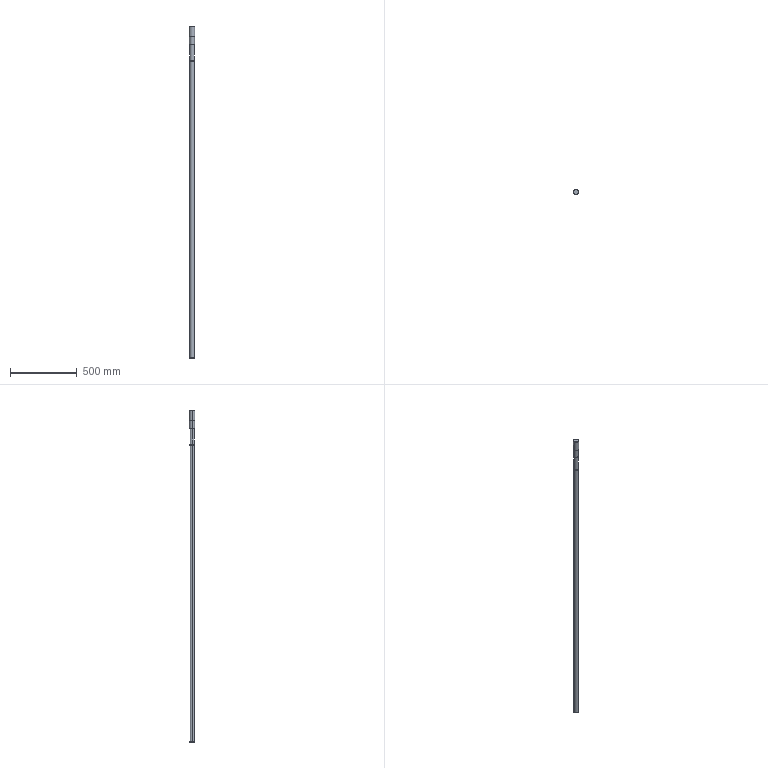Part | SolidWorks | features Chamfer 6, ICE 6, Extrusion 1, MoveFace 1 | 2 solids | 41 faces | box 40 x 40 x 2490 mm | volume 2423592 mm3 | cone 16 | cylinder 15 | plane 10 | commonest cylinder face diameters 16 x4 35 x4 12 x3 38 x2 40 x2
STEP:
#1=CARTESIAN_POINT('',(-7.5,0.,946.05));
#2=VERTEX_POINT('',#1);
#3=CARTESIAN_POINT('',(7.5,0.,946.05));
#4=VERTEX_POINT('',#3);
#5=CARTESIAN_POINT('',(0.,0.,946.05));
#6=DIRECTION('',(0.,0.,-1.));
#7=DIRECTION('',(-1.,0.,0.));
#8=AXIS2_PLACEMENT_3D('',#5,#6,#7);
#9=CIRCLE('',#8,7.5);
#10=EDGE_CURVE('',#2,#4,#9,.T.);
#11=ORIENTED_EDGE('',*,*,#10,.F.);
#12=CARTESIAN_POINT('',(-8.,0.,946.55));
#13=VERTEX_POINT('',#12);
#14=CARTESIAN_POINT('',(-7.5,0.,946.05));
#15=DIRECTION('',(-0.7071,0.,0.7071));
#16=VECTOR('',#15,1000.);
#17=LINE('',#14,#16);
#18=EDGE_CURVE('',#2,#13,#17,.T.);
#19=ORIENTED_EDGE('',*,*,#18,.T.);
#20=CARTESIAN_POINT('',(8.,0.,946.55));
#21=VERTEX_POINT('',#20);
#22=CARTESIAN_POINT('',(0.,0.,946.55));
#23=DIRECTION('',(0.,0.,1.));
#24=DIRECTION('',(-1.,0.,0.));
#25=AXIS2_PLACEMENT_3D('',#22,#23,#24);
#26=CIRCLE('',#25,8.);
#27=EDGE_CURVE('',#21,#13,#26,.T.);
#28=ORIENTED_EDGE('',*,*,#27,.F.);
#29=CARTESIAN_POINT('',(7.5,0.,946.05));
#30=DIRECTION('',(0.7071,0.,0.7071));
#31=VECTOR('',#30,1000.);
#32=LINE('',#29,#31);
#33=EDGE_CURVE('',#4,#21,#32,.T.);
#34=ORIENTED_EDGE('',*,*,#33,.F.);
#35=EDGE_LOOP('',(#11,#19,#28,#34));
#36=FACE_OUTER_BOUND('',#35,.T.);
#37=CARTESIAN_POINT('',(0.,0.,946.05));
#38=DIRECTION('',(0.,0.,1.));
#39=DIRECTION('',(1.,0.,0.));
#40=AXIS2_PLACEMENT_3D('',#37,#38,#39);
#41=CONICAL_SURFACE('',#40,7.5,0.7854);
#42=ADVANCED_FACE('',(#36),#41,.T.);
#43=CARTESIAN_POINT('',(-8.,0.,984.55));
#44=VERTEX_POINT('',#43);
#45=CARTESIAN_POINT('',(8.,0.,984.55));
#46=VERTEX_POINT('',#45);
#47=CARTESIAN_POINT('',(0.,0.,984.55));
#48=DIRECTION('',(0.,0.,-1.));
#49=DIRECTION('',(1.,0.,0.));
#50=AXIS2_PLACEMENT_3D('',#47,#48,#49);
#51=CIRCLE('',#50,8.);
#52=EDGE_CURVE('',#44,#46,#51,.T.);
#53=ORIENTED_EDGE('',*,*,#52,.F.);
#54=CARTESIAN_POINT('',(-8.5,0.,985.05));
#55=VERTEX_POINT('',#54);
#56=CARTESIAN_POINT('',(-8.,0.,984.55));
#57=DIRECTION('',(-0.7071,0.,0.7071));
#58=VECTOR('',#57,1000.);
#59=LINE('',#56,#58);
#60=EDGE_CURVE('',#44,#55,#59,.T.);
#61=ORIENTED_EDGE('',*,*,#60,.T.);
#62=CARTESIAN_POINT('',(8.5,0.,985.05));
#63=VERTEX_POINT('',#62);
#64=CARTESIAN_POINT('',(0.,0.,985.05));
#65=DIRECTION('',(0.,0.,1.));
#66=DIRECTION('',(1.,0.,0.));
#67=AXIS2_PLACEMENT_3D('',#64,#65,#66);
#68=CIRCLE('',#67,8.5);
#69=EDGE_CURVE('',#63,#55,#68,.T.);
#70=ORIENTED_EDGE('',*,*,#69,.F.);
#71=CARTESIAN_POINT('',(8.,0.,984.55));
#72=DIRECTION('',(0.7071,0.,0.7071));
#73=VECTOR('',#72,1000.);
#74=LINE('',#71,#73);
#75=EDGE_CURVE('',#46,#63,#74,.T.);
#76=ORIENTED_EDGE('',*,*,#75,.F.);
#77=EDGE_LOOP('',(#53,#61,#70,#76));
#78=FACE_OUTER_BOUND('',#77,.T.);
#79=CARTESIAN_POINT('',(0.,0.,984.55));
#80=DIRECTION('',(0.,0.,1.));
#81=DIRECTION('',(1.,0.,0.));
#82=AXIS2_PLACEMENT_3D('',#79,#80,#81);
#83=CONICAL_SURFACE('',#82,8.,0.7854);
#84=ADVANCED_FACE('',(#78),#83,.T.);
#85=ORIENTED_EDGE('',*,*,#27,.T.);
#86=CARTESIAN_POINT('',(-8.,0.,946.05));
#87=DIRECTION('',(0.,0.,1.));
#88=VECTOR('',#87,1000.);
#89=LINE('',#86,#88);
#90=EDGE_CURVE('',#13,#44,#89,.T.);
#91=ORIENTED_EDGE('',*,*,#90,.T.);
#92=ORIENTED_EDGE('',*,*,#52,.T.);
#93=CARTESIAN_POINT('',(8.,0.,946.05));
#94=DIRECTION('',(0.,0.,1.));
#95=VECTOR('',#94,1000.);
#96=LINE('',#93,#95);
#97=EDGE_CURVE('',#21,#46,#96,.T.);
#98=ORIENTED_EDGE('',*,*,#97,.F.);
#99=EDGE_LOOP('',(#85,#91,#92,#98));
#100=FACE_OUTER_BOUND('',#99,.T.);
#101=CARTESIAN_POINT('',(0.,0.,946.05));
#102=DIRECTION('',(0.,0.,1.));
#103=DIRECTION('',(1.,0.,0.));
#104=AXIS2_PLACEMENT_3D('',#101,#102,#103);
#105=CYLINDRICAL_SURFACE('',#104,8.);
#106=ADVANCED_FACE('',(#100),#105,.T.);
#107=CARTESIAN_POINT('',(-13.5,0.,985.05));
#108=VERTEX_POINT('',#107);
#109=CARTESIAN_POINT('',(13.5,0.,985.05));
#110=VERTEX_POINT('',#109);
#111=CARTESIAN_POINT('',(0.,0.,985.05));
#112=DIRECTION('',(0.,0.,-1.));
#113=DIRECTION('',(1.,0.,0.));
#114=AXIS2_PLACEMENT_3D('',#111,#112,#113);
#115=CIRCLE('',#114,13.5);
#116=EDGE_CURVE('',#108,#110,#115,.T.);
#117=ORIENTED_EDGE('',*,*,#116,.F.);
#118=CARTESIAN_POINT('',(-17.5,0.,989.05));
#119=VERTEX_POINT('',#118);
#120=CARTESIAN_POINT('',(-17.5,0.,989.05));
#121=DIRECTION('',(-0.7071,0.,0.7071));
#122=VECTOR('',#121,1000.);
#123=LINE('',#120,#122);
#124=EDGE_CURVE('',#108,#119,#123,.T.);
#125=ORIENTED_EDGE('',*,*,#124,.T.);
#126=CARTESIAN_POINT('',(17.5,0.,989.05));
#127=VERTEX_POINT('',#126);
#128=CARTESIAN_POINT('',(0.,0.,989.05));
#129=DIRECTION('',(0.,0.,1.));
#130=DIRECTION('',(1.,0.,0.));
#131=AXIS2_PLACEMENT_3D('',#128,#129,#130);
#132=CIRCLE('',#131,17.5);
#133=EDGE_CURVE('',#127,#119,#132,.T.);
#134=ORIENTED_EDGE('',*,*,#133,.F.);
#135=CARTESIAN_POINT('',(17.5,0.,989.05));
#136=DIRECTION('',(0.7071,0.,0.7071));
#137=VECTOR('',#136,1000.);
#138=LINE('',#135,#137);
#139=EDGE_CURVE('',#110,#127,#138,.T.);
#140=ORIENTED_EDGE('',*,*,#139,.F.);
#141=EDGE_LOOP('',(#117,#125,#134,#140));
#142=FACE_OUTER_BOUND('',#141,.T.);
#143=CARTESIAN_POINT('',(0.,0.,989.05));
#144=DIRECTION('',(0.,0.,1.));
#145=DIRECTION('',(1.,0.,0.));
#146=AXIS2_PLACEMENT_3D('',#143,#144,#145);
#147=CONICAL_SURFACE('',#146,17.5,0.7854);
#148=ADVANCED_FACE('',(#142),#147,.T.);
#149=CARTESIAN_POINT('',(0.,20.,1170.));
#150=VERTEX_POINT('',#149);
#151=CARTESIAN_POINT('',(6.,19.079,1176.));
#152=VERTEX_POINT('',#151);
#153=CARTESIAN_POINT('',(0.,20.,1170.));
#154=CARTESIAN_POINT('',(0.3936,20.,1170.));
#155=CARTESIAN_POINT('',(0.7934,19.988,1170.04));
#156=CARTESIAN_POINT('',(1.564,19.942,1170.194));
#157=CARTESIAN_POINT('',(1.939,19.909,1170.308));
#158=CARTESIAN_POINT('',(2.668,19.825,1170.611));
#159=CARTESIAN_POINT('',(3.015,19.774,1170.798));
#160=CARTESIAN_POINT('',(3.5,19.692,1171.123));
#161=CARTESIAN_POINT('',(3.657,19.664,1171.239));
#162=CARTESIAN_POINT('',(3.959,19.605,1171.487));
#163=CARTESIAN_POINT('',(4.105,19.575,1171.62));
#164=CARTESIAN_POINT('',(4.52,19.485,1172.035));
#165=CARTESIAN_POINT('',(4.766,19.425,1172.335));
#166=CARTESIAN_POINT('',(5.201,19.313,1172.982));
#167=CARTESIAN_POINT('',(5.389,19.261,1173.333));
#168=CARTESIAN_POINT('',(5.69,19.174,1174.055));
#169=CARTESIAN_POINT('',(5.804,19.139,1174.429));
#170=CARTESIAN_POINT('',(5.96,19.092,1175.203));
#171=CARTESIAN_POINT('',(6.,19.079,1175.601));
#172=CARTESIAN_POINT('',(6.,19.079,1176.));
#173=B_SPLINE_CURVE_WITH_KNOTS('',3,(#153,#154,#155,#156,#157,#158,#159,#160,#161,#162,#163,#164,#165,#166,#167,#168,#169,#170,#171,#172),.UNSPECIFIED.,.F.,.F.,(4,2,2,2,2,2,2,2,2,4),(0.009436,0.01061,0.01179,0.01297,0.01356,0.01415,0.01533,0.0165,0.01768,0.01886),.UNSPECIFIED.);
#174=EDGE_CURVE('',#150,#152,#173,.T.);
#175=ORIENTED_EDGE('',*,*,#174,.F.);
#176=CARTESIAN_POINT('',(0.,15.,1170.));
#177=VERTEX_POINT('',#176);
#178=CARTESIAN_POINT('',(0.,65.,1170.));
#179=DIRECTION('',(0.,-1.,0.));
#180=VECTOR('',#179,1000.);
#181=LINE('',#178,#180);
#182=EDGE_CURVE('',#150,#177,#181,.T.);
#183=ORIENTED_EDGE('',*,*,#182,.T.);
#184=CARTESIAN_POINT('',(6.,15.,1176.));
#185=VERTEX_POINT('',#184);
#186=CARTESIAN_POINT('',(0.,15.,1176.));
#187=DIRECTION('',(0.,1.,0.));
#188=DIRECTION('',(0.,0.,1.));
#189=AXIS2_PLACEMENT_3D('',#186,#187,#188);
#190=CIRCLE('',#189,6.);
#191=EDGE_CURVE('',#185,#177,#190,.T.);
#192=ORIENTED_EDGE('',*,*,#191,.F.);
#193=CARTESIAN_POINT('',(6.,65.,1176.));
#194=DIRECTION('',(0.,-1.,0.));
#195=VECTOR('',#194,1000.);
#196=LINE('',#193,#195);
#197=EDGE_CURVE('',#152,#185,#196,.T.);
#198=ORIENTED_EDGE('',*,*,#197,.F.);
#199=EDGE_LOOP('',(#175,#183,#192,#198));
#200=FACE_OUTER_BOUND('',#199,.T.);
#201=CARTESIAN_POINT('',(0.,65.,1176.));
#202=DIRECTION('',(0.,-1.,0.));
#203=DIRECTION('',(0.,0.,-1.));
#204=AXIS2_PLACEMENT_3D('',#201,#202,#203);
#205=CYLINDRICAL_SURFACE('',#204,6.);
#206=ADVANCED_FACE('',(#200),#205,.F.);
#207=CARTESIAN_POINT('',(19.,0.,1245.));
#208=VERTEX_POINT('',#207);
#209=CARTESIAN_POINT('',(-19.,0.,1245.));
#210=VERTEX_POINT('',#209);
#211=CARTESIAN_POINT('',(0.,0.,1245.));
#212=DIRECTION('',(0.,0.,1.));
#213=DIRECTION('',(1.,0.,0.));
#214=AXIS2_PLACEMENT_3D('',#211,#212,#213);
#215=CIRCLE('',#214,19.);
#216=EDGE_CURVE('',#208,#210,#215,.T.);
#217=ORIENTED_EDGE('',*,*,#216,.F.);
#218=CARTESIAN_POINT('',(20.,0.,1244.));
#219=VERTEX_POINT('',#218);
#220=CARTESIAN_POINT('',(19.,0.,1245.));
#221=DIRECTION('',(0.7071,0.,-0.7071));
#222=VECTOR('',#221,1000.);
#223=LINE('',#220,#222);
#224=EDGE_CURVE('',#208,#219,#223,.T.);
#225=ORIENTED_EDGE('',*,*,#224,.T.);
#226=CARTESIAN_POINT('',(-20.,0.,1244.));
#227=VERTEX_POINT('',#226);
#228=CARTESIAN_POINT('',(0.,0.,1244.));
#229=DIRECTION('',(0.,0.,-1.));
#230=DIRECTION('',(1.,0.,0.));
#231=AXIS2_PLACEMENT_3D('',#228,#229,#230);
#232=CIRCLE('',#231,20.);
#233=EDGE_CURVE('',#227,#219,#232,.T.);
#234=ORIENTED_EDGE('',*,*,#233,.F.);
#235=CARTESIAN_POINT('',(-19.,0.,1245.));
#236=DIRECTION('',(-0.7071,0.,-0.7071));
#237=VECTOR('',#236,1000.);
#238=LINE('',#235,#237);
#239=EDGE_CURVE('',#210,#227,#238,.T.);
#240=ORIENTED_EDGE('',*,*,#239,.F.);
#241=EDGE_LOOP('',(#217,#225,#234,#240));
#242=FACE_OUTER_BOUND('',#241,.T.);
#243=CARTESIAN_POINT('',(0.,0.,1245.));
#244=DIRECTION('',(0.,0.,-1.));
#245=DIRECTION('',(-1.,0.,0.));
#246=AXIS2_PLACEMENT_3D('',#243,#244,#245);
#247=CONICAL_SURFACE('',#246,19.,0.7854);
#248=ADVANCED_FACE('',(#242),#247,.T.);
#249=CARTESIAN_POINT('',(19.,0.,1165.));
#250=VERTEX_POINT('',#249);
#251=CARTESIAN_POINT('',(-19.,0.,1165.));
#252=VERTEX_POINT('',#251);
#253=CARTESIAN_POINT('',(0.,0.,1165.));
#254=DIRECTION('',(0.,0.,1.));
#255=DIRECTION('',(1.,0.,0.));
#256=AXIS2_PLACEMENT_3D('',#253,#254,#255);
#257=CIRCLE('',#256,19.);
#258=EDGE_CURVE('',#250,#252,#257,.T.);
#259=ORIENTED_EDGE('',*,*,#258,.T.);
#260=CARTESIAN_POINT('',(-20.,0.,1166.));
#261=VERTEX_POINT('',#260);
#262=CARTESIAN_POINT('',(-20.,0.,1166.));
#263=DIRECTION('',(-0.7071,0.,0.7071));
#264=VECTOR('',#263,1000.);
#265=LINE('',#262,#264);
#266=EDGE_CURVE('',#252,#261,#265,.T.);
#267=ORIENTED_EDGE('',*,*,#266,.T.);
#268=CARTESIAN_POINT('',(20.,0.,1166.));
#269=VERTEX_POINT('',#268);
#270=CARTESIAN_POINT('',(0.,0.,1166.));
#271=DIRECTION('',(0.,0.,1.));
#272=DIRECTION('',(1.,0.,0.));
#273=AXIS2_PLACEMENT_3D('',#270,#271,#272);
#274=CIRCLE('',#273,20.);
#275=EDGE_CURVE('',#269,#261,#274,.T.);
#276=ORIENTED_EDGE('',*,*,#275,.F.);
#277=CARTESIAN_POINT('',(20.,0.,1166.));
#278=DIRECTION('',(0.7071,0.,0.7071));
#279=VECTOR('',#278,1000.);
#280=LINE('',#277,#279);
#281=EDGE_CURVE('',#250,#269,#280,.T.);
#282=ORIENTED_EDGE('',*,*,#281,.F.);
#283=EDGE_LOOP('',(#259,#267,#276,#282));
#284=FACE_OUTER_BOUND('',#283,.T.);
#285=CARTESIAN_POINT('',(0.,0.,1166.));
#286=DIRECTION('',(0.,0.,1.));
#287=DIRECTION('',(1.,0.,0.));
#288=AXIS2_PLACEMENT_3D('',#285,#286,#287);
#289=CONICAL_SURFACE('',#288,20.,0.7854);
#290=ADVANCED_FACE('',(#284),#289,.T.);
#291=ORIENTED_EDGE('',*,*,#258,.F.);
#292=CARTESIAN_POINT('',(19.,0.,1105.));
#293=VERTEX_POINT('',#292);
#294=CARTESIAN_POINT('',(19.,0.,1169.));
#295=DIRECTION('',(0.,0.,-1.));
#296=VECTOR('',#295,1000.);
#297=LINE('',#294,#296);
#298=EDGE_CURVE('',#250,#293,#297,.T.);
#299=ORIENTED_EDGE('',*,*,#298,.T.);
#300=CARTESIAN_POINT('',(-19.,0.,1105.));
#301=VERTEX_POINT('',#300);
#302=CARTESIAN_POINT('',(0.,0.,1105.));
#303=DIRECTION('',(0.,0.,1.));
#304=DIRECTION('',(1.,0.,0.));
#305=AXIS2_PLACEMENT_3D('',#302,#303,#304);
#306=CIRCLE('',#305,19.);
#307=EDGE_CURVE('',#293,#301,#306,.T.);
#308=ORIENTED_EDGE('',*,*,#307,.T.);
#309=CARTESIAN_POINT('',(-19.,0.,1169.));
#310=DIRECTION('',(0.,0.,-1.));
#311=VECTOR('',#310,1000.);
#312=LINE('',#309,#311);
#313=EDGE_CURVE('',#252,#301,#312,.T.);
#314=ORIENTED_EDGE('',*,*,#313,.F.);
#315=EDGE_LOOP('',(#291,#299,#308,#314));
#316=FACE_OUTER_BOUND('',#315,.T.);
#317=CARTESIAN_POINT('',(0.,0.,1169.));
#318=DIRECTION('',(0.,0.,-1.));
#319=DIRECTION('',(-1.,0.,0.));
#320=AXIS2_PLACEMENT_3D('',#317,#318,#319);
#321=CYLINDRICAL_SURFACE('',#320,19.);
#322=ADVANCED_FACE('',(#316),#321,.T.);
#323=CARTESIAN_POINT('',(-6.,19.079,1236.));
#324=VERTEX_POINT('',#323);
#325=CARTESIAN_POINT('',(-6.,19.079,1176.));
#326=VERTEX_POINT('',#325);
#327=CARTESIAN_POINT('',(-6.,19.079,1165.));
#328=DIRECTION('',(0.,0.,-1.));
#329=VECTOR('',#328,1000.);
#330=LINE('',#327,#329);
#331=EDGE_CURVE('',#324,#326,#330,.T.);
#332=ORIENTED_EDGE('',*,*,#331,.T.);
#333=CARTESIAN_POINT('',(-6.,19.079,1176.));
#334=CARTESIAN_POINT('',(-6.,19.079,1175.601));
#335=CARTESIAN_POINT('',(-5.961,19.091,1175.209));
#336=CARTESIAN_POINT('',(-5.845,19.127,1174.631));
#337=CARTESIAN_POINT('',(-5.797,19.141,1174.441));
#338=CARTESIAN_POINT('',(-5.682,19.176,1174.062));
#339=CARTESIAN_POINT('',(-5.615,19.196,1173.875));
#340=CARTESIAN_POINT('',(-5.388,19.261,1173.331));
#341=CARTESIAN_POINT('',(-5.203,19.313,1172.987));
#342=CARTESIAN_POINT('',(-4.877,19.397,1172.499));
#343=CARTESIAN_POINT('',(-4.759,19.426,1172.34));
#344=CARTESIAN_POINT('',(-4.51,19.485,1172.037));
#345=CARTESIAN_POINT('',(-4.378,19.515,1171.893));
#346=CARTESIAN_POINT('',(-3.966,19.605,1171.481));
#347=CARTESIAN_POINT('',(-3.665,19.664,1171.233));
#348=CARTESIAN_POINT('',(-3.009,19.775,1170.794));
#349=CARTESIAN_POINT('',(-2.664,19.825,1170.609));
#350=CARTESIAN_POINT('',(-2.122,19.888,1170.385));
#351=CARTESIAN_POINT('',(-1.938,19.907,1170.318));
#352=CARTESIAN_POINT('',(-1.561,19.94,1170.203));
#353=CARTESIAN_POINT('',(-1.367,19.954,1170.154));
#354=CARTESIAN_POINT('',(-0.7852,19.988,1170.038));
#355=CARTESIAN_POINT('',(-0.3941,20.,1170.));
#356=CARTESIAN_POINT('',(0.,20.,1170.));
#357=B_SPLINE_CURVE_WITH_KNOTS('',3,(#333,#334,#335,#336,#337,#338,#339,#340,#341,#342,#343,#344,#345,#346,#347,#348,#349,#350,#351,#352,#353,#354,#355,#356),.UNSPECIFIED.,.F.,.F.,(4,2,2,2,2,2,2,2,2,2,2,4),(0.,0.00118,0.001769,0.002359,0.003539,0.004128,0.004718,0.005898,0.007077,0.007667,0.008257,0.009436),.UNSPECIFIED.);
#358=EDGE_CURVE('',#326,#150,#357,.T.);
#359=ORIENTED_EDGE('',*,*,#358,.T.);
#360=ORIENTED_EDGE('',*,*,#174,.T.);
#361=CARTESIAN_POINT('',(6.,19.079,1236.));
#362=VERTEX_POINT('',#361);
#363=CARTESIAN_POINT('',(6.,19.079,1165.));
#364=DIRECTION('',(0.,0.,1.));
#365=VECTOR('',#364,1000.);
#366=LINE('',#363,#365);
#367=EDGE_CURVE('',#152,#362,#366,.T.);
#368=ORIENTED_EDGE('',*,*,#367,.T.);
#369=CARTESIAN_POINT('',(6.,19.079,1236.));
#370=CARTESIAN_POINT('',(6.,19.079,1236.399));
#371=CARTESIAN_POINT('',(5.961,19.091,1236.79));
#372=CARTESIAN_POINT('',(5.845,19.127,1237.368));
#373=CARTESIAN_POINT('',(5.797,19.141,1237.558));
#374=CARTESIAN_POINT('',(5.682,19.176,1237.936));
#375=CARTESIAN_POINT('',(5.615,19.196,1238.124));
#376=CARTESIAN_POINT('',(5.389,19.261,1238.668));
#377=CARTESIAN_POINT('',(5.204,19.312,1239.011));
#378=CARTESIAN_POINT('',(4.878,19.396,1239.499));
#379=CARTESIAN_POINT('',(4.76,19.426,1239.658));
#380=CARTESIAN_POINT('',(4.511,19.485,1239.961));
#381=CARTESIAN_POINT('',(4.38,19.515,1240.105));
#382=CARTESIAN_POINT('',(3.968,19.604,1240.517));
#383=CARTESIAN_POINT('',(3.668,19.664,1240.765));
#384=CARTESIAN_POINT('',(3.013,19.775,1241.204));
#385=CARTESIAN_POINT('',(2.667,19.825,1241.389));
#386=CARTESIAN_POINT('',(2.127,19.887,1241.614));
#387=CARTESIAN_POINT('',(1.942,19.906,1241.68));
#388=CARTESIAN_POINT('',(1.566,19.94,1241.795));
#389=CARTESIAN_POINT('',(1.372,19.954,1241.844));
#390=CARTESIAN_POINT('',(0.7905,19.988,1241.961));
#391=CARTESIAN_POINT('',(0.3997,20.,1242.));
#392=CARTESIAN_POINT('',(-0.3879,20.,1242.));
#393=CARTESIAN_POINT('',(-0.788,19.988,1241.961));
#394=CARTESIAN_POINT('',(-1.559,19.943,1241.807));
#395=CARTESIAN_POINT('',(-1.935,19.91,1241.693));
#396=CARTESIAN_POINT('',(-2.482,19.846,1241.466));
#397=CARTESIAN_POINT('',(-2.661,19.823,1241.381));
#398=CARTESIAN_POINT('',(-3.006,19.774,1241.196));
#399=CARTESIAN_POINT('',(-3.173,19.747,1241.096));
#400=CARTESIAN_POINT('',(-3.497,19.693,1240.879));
#401=CARTESIAN_POINT('',(-3.654,19.664,1240.763));
#402=CARTESIAN_POINT('',(-3.956,19.605,1240.515));
#403=CARTESIAN_POINT('',(-4.103,19.575,1240.382));
#404=CARTESIAN_POINT('',(-4.518,19.485,1239.967));
#405=CARTESIAN_POINT('',(-4.765,19.425,1239.667));
#406=CARTESIAN_POINT('',(-5.2,19.314,1239.019));
#407=CARTESIAN_POINT('',(-5.388,19.261,1238.668));
#408=CARTESIAN_POINT('',(-5.689,19.174,1237.946));
#409=CARTESIAN_POINT('',(-5.804,19.14,1237.572));
#410=CARTESIAN_POINT('',(-5.96,19.092,1236.798));
#411=CARTESIAN_POINT('',(-6.,19.079,1236.399));
#412=CARTESIAN_POINT('',(-6.,19.079,1236.));
#413=B_SPLINE_CURVE_WITH_KNOTS('',3,(#369,#370,#371,#372,#373,#374,#375,#376,#377,#378,#379,#380,#381,#382,#383,#384,#385,#386,#387,#388,#389,#390,#391,#392,#393,#394,#395,#396,#397,#398,#399,#400,#401,#402,#403,#404,#405,#406,#407,#408,#409,#410,#411,#412),.UNSPECIFIED.,.F.,.F.,(4,2,2,2,2,2,2,2,2,2,2,2,2,2,2,2,2,2,2,2,2,4),(0.,0.001179,0.001768,0.002358,0.003536,0.004126,0.004715,0.005894,0.007073,0.007662,0.008252,0.009431,0.01061,0.01179,0.01238,0.01297,0.01356,0.01415,0.01532,0.0165,0.01768,0.01886),.UNSPECIFIED.);
#414=EDGE_CURVE('',#362,#324,#413,.T.);
#415=ORIENTED_EDGE('',*,*,#414,.T.);
#416=EDGE_LOOP('',(#332,#359,#360,#368,#415));
#417=FACE_BOUND('',#416,.T.);
#418=ORIENTED_EDGE('',*,*,#275,.T.);
#419=CARTESIAN_POINT('',(-20.,0.,1165.));
#420=DIRECTION('',(0.,0.,1.));
#421=VECTOR('',#420,1000.);
#422=LINE('',#419,#421);
#423=EDGE_CURVE('',#261,#227,#422,.T.);
#424=ORIENTED_EDGE('',*,*,#423,.T.);
#425=ORIENTED_EDGE('',*,*,#233,.T.);
#426=CARTESIAN_POINT('',(20.,0.,1165.));
#427=DIRECTION('',(0.,0.,1.));
#428=VECTOR('',#427,1000.);
#429=LINE('',#426,#428);
#430=EDGE_CURVE('',#269,#219,#429,.T.);
#431=ORIENTED_EDGE('',*,*,#430,.F.);
#432=EDGE_LOOP('',(#418,#424,#425,#431));
#433=FACE_OUTER_BOUND('',#432,.T.);
#434=CARTESIAN_POINT('',(0.,0.,1165.));
#435=DIRECTION('',(0.,0.,1.));
#436=DIRECTION('',(1.,0.,0.));
#437=AXIS2_PLACEMENT_3D('',#434,#435,#436);
#438=CYLINDRICAL_SURFACE('',#437,20.);
#439=ADVANCED_FACE('',(#417,#433),#438,.T.);
#440=CARTESIAN_POINT('',(17.5,0.,1105.));
#441=VERTEX_POINT('',#440);
#442=CARTESIAN_POINT('',(-17.5,0.,1105.));
#443=VERTEX_POINT('',#442);
#444=CARTESIAN_POINT('',(0.,0.,1105.));
#445=DIRECTION('',(0.,0.,1.));
#446=DIRECTION('',(1.,0.,0.));
#447=AXIS2_PLACEMENT_3D('',#444,#445,#446);
#448=CIRCLE('',#447,17.5);
#449=EDGE_CURVE('',#441,#443,#448,.T.);
#450=ORIENTED_EDGE('',*,*,#449,.F.);
#451=CARTESIAN_POINT('',(17.5,0.,1245.));
#452=DIRECTION('',(0.,0.,-1.));
#453=VECTOR('',#452,1000.);
#454=LINE('',#451,#453);
#455=EDGE_CURVE('',#441,#127,#454,.T.);
#456=ORIENTED_EDGE('',*,*,#455,.T.);
#457=ORIENTED_EDGE('',*,*,#133,.T.);
#458=CARTESIAN_POINT('',(-17.5,0.,1245.));
#459=DIRECTION('',(0.,0.,-1.));
#460=VECTOR('',#459,1000.);
#461=LINE('',#458,#460);
#462=EDGE_CURVE('',#443,#119,#461,.T.);
#463=ORIENTED_EDGE('',*,*,#462,.F.);
#464=EDGE_LOOP('',(#450,#456,#457,#463));
#465=FACE_OUTER_BOUND('',#464,.T.);
#466=CARTESIAN_POINT('',(0.,0.,1245.));
#467=DIRECTION('',(0.,0.,-1.));
#468=DIRECTION('',(-1.,0.,0.));
#469=AXIS2_PLACEMENT_3D('',#466,#467,#468);
#470=CYLINDRICAL_SURFACE('',#469,17.5);
#471=ADVANCED_FACE('',(#465),#470,.T.);
#472=ORIENTED_EDGE('',*,*,#455,.F.);
#473=CARTESIAN_POINT('',(0.,0.,1105.));
#474=DIRECTION('',(0.,0.,1.));
#475=DIRECTION('',(1.,0.,0.));
#476=AXIS2_PLACEMENT_3D('',#473,#474,#475);
#477=CIRCLE('',#476,17.5);
#478=EDGE_CURVE('',#443,#441,#477,.T.);
#479=ORIENTED_EDGE('',*,*,#478,.F.);
#480=ORIENTED_EDGE('',*,*,#462,.T.);
#481=CARTESIAN_POINT('',(0.,0.,989.05));
#482=DIRECTION('',(0.,0.,1.));
#483=DIRECTION('',(1.,0.,0.));
#484=AXIS2_PLACEMENT_3D('',#481,#482,#483);
#485=CIRCLE('',#484,17.5);
#486=EDGE_CURVE('',#119,#127,#485,.T.);
#487=ORIENTED_EDGE('',*,*,#486,.T.);
#488=EDGE_LOOP('',(#472,#479,#480,#487));
#489=FACE_OUTER_BOUND('',#488,.T.);
#490=CARTESIAN_POINT('',(0.,0.,1245.));
#491=DIRECTION('',(0.,0.,-1.));
#492=DIRECTION('',(-1.,0.,0.));
#493=AXIS2_PLACEMENT_3D('',#490,#491,#492);
#494=CYLINDRICAL_SURFACE('',#493,17.5);
#495=ADVANCED_FACE('',(#489),#494,.T.);
#496=ORIENTED_EDGE('',*,*,#423,.F.);
#497=CARTESIAN_POINT('',(0.,0.,1166.));
#498=DIRECTION('',(0.,0.,1.));
#499=DIRECTION('',(1.,0.,0.));
#500=AXIS2_PLACEMENT_3D('',#497,#498,#499);
#501=CIRCLE('',#500,20.);
#502=EDGE_CURVE('',#261,#269,#501,.T.);
#503=ORIENTED_EDGE('',*,*,#502,.T.);
#504=ORIENTED_EDGE('',*,*,#430,.T.);
#505=CARTESIAN_POINT('',(0.,0.,1244.));
#506=DIRECTION('',(0.,0.,-1.));
#507=DIRECTION('',(1.,0.,0.));
#508=AXIS2_PLACEMENT_3D('',#505,#506,#507);
#509=CIRCLE('',#508,20.);
#510=EDGE_CURVE('',#219,#227,#509,.T.);
#511=ORIENTED_EDGE('',*,*,#510,.T.);
#512=EDGE_LOOP('',(#496,#503,#504,#511));
#513=FACE_OUTER_BOUND('',#512,.T.);
#514=CARTESIAN_POINT('',(0.,0.,1165.));
#515=DIRECTION('',(0.,0.,1.));
#516=DIRECTION('',(1.,0.,0.));
#517=AXIS2_PLACEMENT_3D('',#514,#515,#516);
#518=CYLINDRICAL_SURFACE('',#517,20.);
#519=ADVANCED_FACE('',(#513),#518,.T.);
#520=ORIENTED_EDGE('',*,*,#298,.F.);
#521=CARTESIAN_POINT('',(0.,0.,1165.));
#522=DIRECTION('',(0.,0.,1.));
#523=DIRECTION('',(1.,0.,0.));
#524=AXIS2_PLACEMENT_3D('',#521,#522,#523);
#525=CIRCLE('',#524,19.);
#526=EDGE_CURVE('',#252,#250,#525,.T.);
#527=ORIENTED_EDGE('',*,*,#526,.F.);
#528=ORIENTED_EDGE('',*,*,#313,.T.);
#529=CARTESIAN_POINT('',(0.,0.,1105.));
#530=DIRECTION('',(0.,0.,1.));
#531=DIRECTION('',(1.,0.,0.));
#532=AXIS2_PLACEMENT_3D('',#529,#530,#531);
#533=CIRCLE('',#532,19.);
#534=EDGE_CURVE('',#301,#293,#533,.T.);
#535=ORIENTED_EDGE('',*,*,#534,.T.);
#536=EDGE_LOOP('',(#520,#527,#528,#535));
#537=FACE_OUTER_BOUND('',#536,.T.);
#538=CARTESIAN_POINT('',(0.,0.,1169.));
#539=DIRECTION('',(0.,0.,-1.));
#540=DIRECTION('',(-1.,0.,0.));
#541=AXIS2_PLACEMENT_3D('',#538,#539,#540);
#542=CYLINDRICAL_SURFACE('',#541,19.);
#543=ADVANCED_FACE('',(#537),#542,.T.);
#544=ORIENTED_EDGE('',*,*,#478,.T.);
#545=ORIENTED_EDGE('',*,*,#449,.T.);
#546=EDGE_LOOP('',(#544,#545));
#547=FACE_BOUND('',#546,.T.);
#548=ORIENTED_EDGE('',*,*,#534,.F.);
#549=ORIENTED_EDGE('',*,*,#307,.F.);
#550=EDGE_LOOP('',(#548,#549));
#551=FACE_OUTER_BOUND('',#550,.T.);
#552=CARTESIAN_POINT('',(0.,0.,1105.));
#553=DIRECTION('',(0.,0.,1.));
#554=DIRECTION('',(1.,0.,0.));
#555=AXIS2_PLACEMENT_3D('',#552,#553,#554);
#556=PLANE('',#555);
#557=ADVANCED_FACE('',(#547,#551),#556,.F.);
#558=CARTESIAN_POINT('',(0.,0.,1245.));
#559=DIRECTION('',(0.,0.,1.));
#560=DIRECTION('',(1.,0.,0.));
#561=AXIS2_PLACEMENT_3D('',#558,#559,#560);
#562=CIRCLE('',#561,19.);
#563=EDGE_CURVE('',#210,#208,#562,.T.);
#564=ORIENTED_EDGE('',*,*,#563,.T.);
#565=ORIENTED_EDGE('',*,*,#216,.T.);
#566=EDGE_LOOP('',(#564,#565));
#567=FACE_OUTER_BOUND('',#566,.T.);
#568=CARTESIAN_POINT('',(0.,0.,1245.));
#569=DIRECTION('',(0.,0.,1.));
#570=DIRECTION('',(1.,0.,0.));
#571=AXIS2_PLACEMENT_3D('',#568,#569,#570);
#572=PLANE('',#571);
#573=ADVANCED_FACE('',(#567),#572,.T.);
#574=ORIENTED_EDGE('',*,*,#266,.F.);
#575=ORIENTED_EDGE('',*,*,#526,.T.);
#576=ORIENTED_EDGE('',*,*,#281,.T.);
#577=ORIENTED_EDGE('',*,*,#502,.F.);
#578=EDGE_LOOP('',(#574,#575,#576,#577));
#579=FACE_OUTER_BOUND('',#578,.T.);
#580=CARTESIAN_POINT('',(0.,0.,1166.));
#581=DIRECTION('',(0.,0.,1.));
#582=DIRECTION('',(1.,0.,0.));
#583=AXIS2_PLACEMENT_3D('',#580,#581,#582);
#584=CONICAL_SURFACE('',#583,20.,0.7854);
#585=ADVANCED_FACE('',(#579),#584,.T.);
#586=ORIENTED_EDGE('',*,*,#224,.F.);
#587=ORIENTED_EDGE('',*,*,#563,.F.);
#588=ORIENTED_EDGE('',*,*,#239,.T.);
#589=ORIENTED_EDGE('',*,*,#510,.F.);
#590=EDGE_LOOP('',(#586,#587,#588,#589));
#591=FACE_OUTER_BOUND('',#590,.T.);
#592=CARTESIAN_POINT('',(0.,0.,1245.));
#593=DIRECTION('',(0.,0.,-1.));
#594=DIRECTION('',(-1.,0.,0.));
#595=AXIS2_PLACEMENT_3D('',#592,#593,#594);
#596=CONICAL_SURFACE('',#595,19.,0.7854);
#597=ADVANCED_FACE('',(#591),#596,.T.);
#598=ORIENTED_EDGE('',*,*,#182,.F.);
#599=ORIENTED_EDGE('',*,*,#358,.F.);
#600=CARTESIAN_POINT('',(-6.,15.,1176.));
#601=VERTEX_POINT('',#600);
#602=CARTESIAN_POINT('',(-6.,65.,1176.));
#603=DIRECTION('',(0.,-1.,0.));
#604=VECTOR('',#603,1000.);
#605=LINE('',#602,#604);
#606=EDGE_CURVE('',#326,#601,#605,.T.);
#607=ORIENTED_EDGE('',*,*,#606,.T.);
#608=CARTESIAN_POINT('',(0.,15.,1176.));
#609=DIRECTION('',(0.,1.,0.));
#610=DIRECTION('',(0.,0.,1.));
#611=AXIS2_PLACEMENT_3D('',#608,#609,#610);
#612=CIRCLE('',#611,6.);
#613=EDGE_CURVE('',#177,#601,#612,.T.);
#614=ORIENTED_EDGE('',*,*,#613,.F.);
#615=EDGE_LOOP('',(#598,#599,#607,#614));
#616=FACE_OUTER_BOUND('',#615,.T.);
#617=CARTESIAN_POINT('',(0.,65.,1176.));
#618=DIRECTION('',(0.,-1.,0.));
#619=DIRECTION('',(0.,0.,-1.));
#620=AXIS2_PLACEMENT_3D('',#617,#618,#619);
#621=CYLINDRICAL_SURFACE('',#620,6.);
#622=ADVANCED_FACE('',(#616),#621,.F.);
#623=CARTESIAN_POINT('',(-6.,15.,1236.));
#624=VERTEX_POINT('',#623);
#625=CARTESIAN_POINT('',(-6.,65.,1236.));
#626=DIRECTION('',(0.,-1.,0.));
#627=VECTOR('',#626,1000.);
#628=LINE('',#625,#627);
#629=EDGE_CURVE('',#324,#624,#628,.T.);
#630=ORIENTED_EDGE('',*,*,#629,.T.);
#631=CARTESIAN_POINT('',(-6.,15.,1176.));
#632=DIRECTION('',(0.,0.,1.));
#633=VECTOR('',#632,1000.);
#634=LINE('',#631,#633);
#635=EDGE_CURVE('',#601,#624,#634,.T.);
#636=ORIENTED_EDGE('',*,*,#635,.F.);
#637=ORIENTED_EDGE('',*,*,#606,.F.);
#638=ORIENTED_EDGE('',*,*,#331,.F.);
#639=EDGE_LOOP('',(#630,#636,#637,#638));
#640=FACE_OUTER_BOUND('',#639,.T.);
#641=CARTESIAN_POINT('',(-6.,65.,1176.));
#642=DIRECTION('',(1.,0.,0.));
#643=DIRECTION('',(0.,0.,-1.));
#644=AXIS2_PLACEMENT_3D('',#641,#642,#643);
#645=PLANE('',#644);
#646=ADVANCED_FACE('',(#640),#645,.T.);
#647=CARTESIAN_POINT('',(6.,15.,1236.));
#648=VERTEX_POINT('',#647);
#649=CARTESIAN_POINT('',(6.,65.,1236.));
#650=DIRECTION('',(0.,-1.,0.));
#651=VECTOR('',#650,1000.);
#652=LINE('',#649,#651);
#653=EDGE_CURVE('',#362,#648,#652,.T.);
#654=ORIENTED_EDGE('',*,*,#653,.T.);
#655=CARTESIAN_POINT('',(0.,15.,1236.));
#656=DIRECTION('',(0.,1.,0.));
#657=DIRECTION('',(0.,0.,1.));
#658=AXIS2_PLACEMENT_3D('',#655,#656,#657);
#659=CIRCLE('',#658,6.);
#660=EDGE_CURVE('',#624,#648,#659,.T.);
#661=ORIENTED_EDGE('',*,*,#660,.F.);
#662=ORIENTED_EDGE('',*,*,#629,.F.);
#663=ORIENTED_EDGE('',*,*,#414,.F.);
#664=EDGE_LOOP('',(#654,#661,#662,#663));
#665=FACE_OUTER_BOUND('',#664,.T.);
#666=CARTESIAN_POINT('',(0.,65.,1236.));
#667=DIRECTION('',(0.,-1.,0.));
#668=DIRECTION('',(0.,0.,-1.));
#669=AXIS2_PLACEMENT_3D('',#666,#667,#668);
#670=CYLINDRICAL_SURFACE('',#669,6.);
#671=ADVANCED_FACE('',(#665),#670,.F.);
#672=ORIENTED_EDGE('',*,*,#197,.T.);
#673=CARTESIAN_POINT('',(6.,15.,1176.));
#674=DIRECTION('',(0.,0.,-1.));
#675=VECTOR('',#674,1000.);
#676=LINE('',#673,#675);
#677=EDGE_CURVE('',#648,#185,#676,.T.);
#678=ORIENTED_EDGE('',*,*,#677,.F.);
#679=ORIENTED_EDGE('',*,*,#653,.F.);
#680=ORIENTED_EDGE('',*,*,#367,.F.);
#681=EDGE_LOOP('',(#672,#678,#679,#680));
#682=FACE_OUTER_BOUND('',#681,.T.);
#683=CARTESIAN_POINT('',(6.,65.,1176.));
#684=DIRECTION('',(-1.,0.,0.));
#685=DIRECTION('',(0.,0.,1.));
#686=AXIS2_PLACEMENT_3D('',#683,#684,#685);
#687=PLANE('',#686);
#688=ADVANCED_FACE('',(#682),#687,.T.);
#689=ORIENTED_EDGE('',*,*,#191,.T.);
#690=ORIENTED_EDGE('',*,*,#613,.T.);
#691=ORIENTED_EDGE('',*,*,#635,.T.);
#692=ORIENTED_EDGE('',*,*,#660,.T.);
#693=ORIENTED_EDGE('',*,*,#677,.T.);
#694=EDGE_LOOP('',(#689,#690,#691,#692,#693));
#695=FACE_OUTER_BOUND('',#694,.T.);
#696=CARTESIAN_POINT('',(0.,15.,1176.));
#697=DIRECTION('',(0.,1.,0.));
#698=DIRECTION('',(0.,0.,1.));
#699=AXIS2_PLACEMENT_3D('',#696,#697,#698);
#700=PLANE('',#699);
#701=ADVANCED_FACE('',(#695),#700,.T.);
#702=ORIENTED_EDGE('',*,*,#69,.T.);
#703=CARTESIAN_POINT('',(0.,0.,985.05));
#704=DIRECTION('',(0.,0.,1.));
#705=DIRECTION('',(1.,0.,0.));
#706=AXIS2_PLACEMENT_3D('',#703,#704,#705);
#707=CIRCLE('',#706,8.5);
#708=EDGE_CURVE('',#55,#63,#707,.T.);
#709=ORIENTED_EDGE('',*,*,#708,.T.);
#710=EDGE_LOOP('',(#702,#709));
#711=FACE_BOUND('',#710,.T.);
#712=CARTESIAN_POINT('',(0.,0.,985.05));
#713=DIRECTION('',(0.,0.,-1.));
#714=DIRECTION('',(1.,0.,0.));
#715=AXIS2_PLACEMENT_3D('',#712,#713,#714);
#716=CIRCLE('',#715,13.5);
#717=EDGE_CURVE('',#110,#108,#716,.T.);
#718=ORIENTED_EDGE('',*,*,#717,.T.);
#719=ORIENTED_EDGE('',*,*,#116,.T.);
#720=EDGE_LOOP('',(#718,#719));
#721=FACE_OUTER_BOUND('',#720,.T.);
#722=CARTESIAN_POINT('',(-24.605,-20.,985.05));
#723=DIRECTION('',(0.,0.,1.));
#724=DIRECTION('',(1.,0.,0.));
#725=AXIS2_PLACEMENT_3D('',#722,#723,#724);
#726=PLANE('',#725);
#727=ADVANCED_FACE('',(#711,#721),#726,.F.);
#728=ORIENTED_EDGE('',*,*,#124,.F.);
#729=ORIENTED_EDGE('',*,*,#717,.F.);
#730=ORIENTED_EDGE('',*,*,#139,.T.);
#731=ORIENTED_EDGE('',*,*,#486,.F.);
#732=EDGE_LOOP('',(#728,#729,#730,#731));
#733=FACE_OUTER_BOUND('',#732,.T.);
#734=CARTESIAN_POINT('',(0.,0.,989.05));
#735=DIRECTION('',(0.,0.,1.));
#736=DIRECTION('',(1.,0.,0.));
#737=AXIS2_PLACEMENT_3D('',#734,#735,#736);
#738=CONICAL_SURFACE('',#737,17.5,0.7854);
#739=ADVANCED_FACE('',(#733),#738,.T.);
#740=ORIENTED_EDGE('',*,*,#90,.F.);
#741=CARTESIAN_POINT('',(0.,0.,946.55));
#742=DIRECTION('',(0.,0.,1.));
#743=DIRECTION('',(-1.,0.,0.));
#744=AXIS2_PLACEMENT_3D('',#741,#742,#743);
#745=CIRCLE('',#744,8.);
#746=EDGE_CURVE('',#13,#21,#745,.T.);
#747=ORIENTED_EDGE('',*,*,#746,.T.);
#748=ORIENTED_EDGE('',*,*,#97,.T.);
#749=CARTESIAN_POINT('',(0.,0.,984.55));
#750=DIRECTION('',(0.,0.,-1.));
#751=DIRECTION('',(1.,0.,0.));
#752=AXIS2_PLACEMENT_3D('',#749,#750,#751);
#753=CIRCLE('',#752,8.);
#754=EDGE_CURVE('',#46,#44,#753,.T.);
#755=ORIENTED_EDGE('',*,*,#754,.T.);
#756=EDGE_LOOP('',(#740,#747,#748,#755));
#757=FACE_OUTER_BOUND('',#756,.T.);
#758=CARTESIAN_POINT('',(0.,0.,946.05));
#759=DIRECTION('',(0.,0.,1.));
#760=DIRECTION('',(1.,0.,0.));
#761=AXIS2_PLACEMENT_3D('',#758,#759,#760);
#762=CYLINDRICAL_SURFACE('',#761,8.);
#763=ADVANCED_FACE('',(#757),#762,.T.);
#764=CARTESIAN_POINT('',(0.,0.,946.05));
#765=DIRECTION('',(0.,0.,-1.));
#766=DIRECTION('',(-1.,0.,0.));
#767=AXIS2_PLACEMENT_3D('',#764,#765,#766);
#768=CIRCLE('',#767,7.5);
#769=EDGE_CURVE('',#4,#2,#768,.T.);
#770=ORIENTED_EDGE('',*,*,#769,.T.);
#771=ORIENTED_EDGE('',*,*,#10,.T.);
#772=EDGE_LOOP('',(#770,#771));
#773=FACE_OUTER_BOUND('',#772,.T.);
#774=CARTESIAN_POINT('',(0.,0.,946.05));
#775=DIRECTION('',(0.,0.,-1.));
#776=DIRECTION('',(-1.,0.,0.));
#777=AXIS2_PLACEMENT_3D('',#774,#775,#776);
#778=PLANE('',#777);
#779=ADVANCED_FACE('',(#773),#778,.T.);
#780=ORIENTED_EDGE('',*,*,#60,.F.);
#781=ORIENTED_EDGE('',*,*,#754,.F.);
#782=ORIENTED_EDGE('',*,*,#75,.T.);
#783=ORIENTED_EDGE('',*,*,#708,.F.);
#784=EDGE_LOOP('',(#780,#781,#782,#783));
#785=FACE_OUTER_BOUND('',#784,.T.);
#786=CARTESIAN_POINT('',(0.,0.,984.55));
#787=DIRECTION('',(0.,0.,1.));
#788=DIRECTION('',(1.,0.,0.));
#789=AXIS2_PLACEMENT_3D('',#786,#787,#788);
#790=CONICAL_SURFACE('',#789,8.,0.7854);
#791=ADVANCED_FACE('',(#785),#790,.T.);
#792=ORIENTED_EDGE('',*,*,#18,.F.);
#793=ORIENTED_EDGE('',*,*,#769,.F.);
#794=ORIENTED_EDGE('',*,*,#33,.T.);
#795=ORIENTED_EDGE('',*,*,#746,.F.);
#796=EDGE_LOOP('',(#792,#793,#794,#795));
#797=FACE_OUTER_BOUND('',#796,.T.);
#798=CARTESIAN_POINT('',(0.,0.,946.05));
#799=DIRECTION('',(0.,0.,1.));
#800=DIRECTION('',(1.,0.,0.));
#801=AXIS2_PLACEMENT_3D('',#798,#799,#800);
#802=CONICAL_SURFACE('',#801,7.5,0.7854);
#803=ADVANCED_FACE('',(#797),#802,.T.);
#804=CLOSED_SHELL('',(#42,#84,#106,#148,#206,#248,#290,#322,#439,#471,#495,#519,#543,#557,#573,#585,#597,#622,#646,#671,#688,#701,#727,#739,#763,#779,#791,#803));
#805=MANIFOLD_SOLID_BREP('',#804);
#806=CARTESIAN_POINT('',(-8.,0.,984.05));
#807=VERTEX_POINT('',#806);
#808=CARTESIAN_POINT('',(8.,0.,984.05));
#809=VERTEX_POINT('',#808);
#810=CARTESIAN_POINT('',(0.,0.,984.05));
#811=DIRECTION('',(0.,0.,1.));
#812=DIRECTION('',(-1.,0.,0.));
#813=AXIS2_PLACEMENT_3D('',#810,#811,#812);
#814=CIRCLE('',#813,8.);
#815=EDGE_CURVE('',#807,#809,#814,.T.);
#816=ORIENTED_EDGE('',*,*,#815,.F.);
#817=CARTESIAN_POINT('',(-9.,0.,985.05));
#818=VERTEX_POINT('',#817);
#819=CARTESIAN_POINT('',(-8.,0.,984.05));
#820=DIRECTION('',(-0.7071,0.,0.7071));
#821=VECTOR('',#820,1000.);
#822=LINE('',#819,#821);
#823=EDGE_CURVE('',#807,#818,#822,.T.);
#824=ORIENTED_EDGE('',*,*,#823,.T.);
#825=CARTESIAN_POINT('',(9.,0.,985.05));
#826=VERTEX_POINT('',#825);
#827=CARTESIAN_POINT('',(0.,0.,985.05));
#828=DIRECTION('',(0.,0.,-1.));
#829=DIRECTION('',(-1.,0.,0.));
#830=AXIS2_PLACEMENT_3D('',#827,#828,#829);
#831=CIRCLE('',#830,9.);
#832=EDGE_CURVE('',#826,#818,#831,.T.);
#833=ORIENTED_EDGE('',*,*,#832,.F.);
#834=CARTESIAN_POINT('',(8.,0.,984.05));
#835=DIRECTION('',(0.7071,0.,0.7071));
#836=VECTOR('',#835,1000.);
#837=LINE('',#834,#836);
#838=EDGE_CURVE('',#809,#826,#837,.T.);
#839=ORIENTED_EDGE('',*,*,#838,.F.);
#840=EDGE_LOOP('',(#816,#824,#833,#839));
#841=FACE_OUTER_BOUND('',#840,.T.);
#842=CARTESIAN_POINT('',(0.,0.,984.05));
#843=DIRECTION('',(0.,0.,1.));
#844=DIRECTION('',(1.,0.,0.));
#845=AXIS2_PLACEMENT_3D('',#842,#843,#844);
#846=CONICAL_SURFACE('',#845,8.,0.7854);
#847=ADVANCED_FACE('',(#841),#846,.F.);
#848=CARTESIAN_POINT('',(-8.,0.,945.05));
#849=VERTEX_POINT('',#848);
#850=CARTESIAN_POINT('',(8.,0.,945.05));
#851=VERTEX_POINT('',#850);
#852=CARTESIAN_POINT('',(0.,0.,945.05));
#853=DIRECTION('',(0.,0.,1.));
#854=DIRECTION('',(1.,0.,0.));
#855=AXIS2_PLACEMENT_3D('',#852,#853,#854);
#856=CIRCLE('',#855,8.);
#857=EDGE_CURVE('',#849,#851,#856,.T.);
#858=ORIENTED_EDGE('',*,*,#857,.F.);
#859=CARTESIAN_POINT('',(-8.,0.,945.05));
#860=DIRECTION('',(0.,0.,1.));
#861=VECTOR('',#860,1000.);
#862=LINE('',#859,#861);
#863=EDGE_CURVE('',#849,#807,#862,.T.);
#864=ORIENTED_EDGE('',*,*,#863,.T.);
#865=ORIENTED_EDGE('',*,*,#815,.T.);
#866=CARTESIAN_POINT('',(8.,0.,945.05));
#867=DIRECTION('',(0.,0.,1.));
#868=VECTOR('',#867,1000.);
#869=LINE('',#866,#868);
#870=EDGE_CURVE('',#851,#809,#869,.T.);
#871=ORIENTED_EDGE('',*,*,#870,.F.);
#872=EDGE_LOOP('',(#858,#864,#865,#871));
#873=FACE_OUTER_BOUND('',#872,.T.);
#874=CARTESIAN_POINT('',(0.,0.,945.05));
#875=DIRECTION('',(0.,0.,1.));
#876=DIRECTION('',(1.,0.,0.));
#877=AXIS2_PLACEMENT_3D('',#874,#875,#876);
#878=CYLINDRICAL_SURFACE('',#877,8.);
#879=ADVANCED_FACE('',(#873),#878,.F.);
#880=CARTESIAN_POINT('',(13.5,0.,985.05));
#881=VERTEX_POINT('',#880);
#882=CARTESIAN_POINT('',(-13.5,0.,985.05));
#883=VERTEX_POINT('',#882);
#884=CARTESIAN_POINT('',(0.,0.,985.05));
#885=DIRECTION('',(0.,0.,1.));
#886=DIRECTION('',(-1.,0.,0.));
#887=AXIS2_PLACEMENT_3D('',#884,#885,#886);
#888=CIRCLE('',#887,13.5);
#889=EDGE_CURVE('',#881,#883,#888,.T.);
#890=ORIENTED_EDGE('',*,*,#889,.F.);
#891=CARTESIAN_POINT('',(17.5,0.,981.05));
#892=VERTEX_POINT('',#891);
#893=CARTESIAN_POINT('',(17.5,0.,981.05));
#894=DIRECTION('',(0.7071,0.,-0.7071));
#895=VECTOR('',#894,1000.);
#896=LINE('',#893,#895);
#897=EDGE_CURVE('',#881,#892,#896,.T.);
#898=ORIENTED_EDGE('',*,*,#897,.T.);
#899=CARTESIAN_POINT('',(-17.5,0.,981.05));
#900=VERTEX_POINT('',#899);
#901=CARTESIAN_POINT('',(0.,0.,981.05));
#902=DIRECTION('',(0.,0.,-1.));
#903=DIRECTION('',(-1.,0.,0.));
#904=AXIS2_PLACEMENT_3D('',#901,#902,#903);
#905=CIRCLE('',#904,17.5);
#906=EDGE_CURVE('',#900,#892,#905,.T.);
#907=ORIENTED_EDGE('',*,*,#906,.F.);
#908=CARTESIAN_POINT('',(-17.5,0.,981.05));
#909=DIRECTION('',(-0.7071,0.,-0.7071));
#910=VECTOR('',#909,1000.);
#911=LINE('',#908,#910);
#912=EDGE_CURVE('',#883,#900,#911,.T.);
#913=ORIENTED_EDGE('',*,*,#912,.F.);
#914=EDGE_LOOP('',(#890,#898,#907,#913));
#915=FACE_OUTER_BOUND('',#914,.T.);
#916=CARTESIAN_POINT('',(0.,0.,981.05));
#917=DIRECTION('',(0.,0.,-1.));
#918=DIRECTION('',(-1.,0.,0.));
#919=AXIS2_PLACEMENT_3D('',#916,#917,#918);
#920=CONICAL_SURFACE('',#919,17.5,0.7854);
#921=ADVANCED_FACE('',(#915),#920,.T.);
#922=ORIENTED_EDGE('',*,*,#906,.T.);
#923=CARTESIAN_POINT('',(17.5,0.,-1244.));
#924=VERTEX_POINT('',#923);
#925=CARTESIAN_POINT('',(17.5,0.,1245.));
#926=DIRECTION('',(0.,0.,-1.));
#927=VECTOR('',#926,1000.);
#928=LINE('',#925,#927);
#929=EDGE_CURVE('',#892,#924,#928,.T.);
#930=ORIENTED_EDGE('',*,*,#929,.T.);
#931=CARTESIAN_POINT('',(-17.5,0.,-1244.));
#932=VERTEX_POINT('',#931);
#933=CARTESIAN_POINT('',(0.,0.,-1244.));
#934=DIRECTION('',(0.,0.,1.));
#935=DIRECTION('',(1.,0.,0.));
#936=AXIS2_PLACEMENT_3D('',#933,#934,#935);
#937=CIRCLE('',#936,17.5);
#938=EDGE_CURVE('',#924,#932,#937,.T.);
#939=ORIENTED_EDGE('',*,*,#938,.T.);
#940=CARTESIAN_POINT('',(-17.5,0.,1245.));
#941=DIRECTION('',(0.,0.,-1.));
#942=VECTOR('',#941,1000.);
#943=LINE('',#940,#942);
#944=EDGE_CURVE('',#900,#932,#943,.T.);
#945=ORIENTED_EDGE('',*,*,#944,.F.);
#946=EDGE_LOOP('',(#922,#930,#939,#945));
#947=FACE_OUTER_BOUND('',#946,.T.);
#948=CARTESIAN_POINT('',(0.,0.,1245.));
#949=DIRECTION('',(0.,0.,-1.));
#950=DIRECTION('',(-1.,0.,0.));
#951=AXIS2_PLACEMENT_3D('',#948,#949,#950);
#952=CYLINDRICAL_SURFACE('',#951,17.5);
#953=ADVANCED_FACE('',(#947),#952,.T.);
#954=CARTESIAN_POINT('',(-16.5,0.,-1245.));
#955=VERTEX_POINT('',#954);
#956=CARTESIAN_POINT('',(16.5,0.,-1245.));
#957=VERTEX_POINT('',#956);
#958=CARTESIAN_POINT('',(0.,0.,-1245.));
#959=DIRECTION('',(0.,0.,-1.));
#960=DIRECTION('',(1.,0.,0.));
#961=AXIS2_PLACEMENT_3D('',#958,#959,#960);
#962=CIRCLE('',#961,16.5);
#963=EDGE_CURVE('',#955,#957,#962,.T.);
#964=ORIENTED_EDGE('',*,*,#963,.F.);
#965=CARTESIAN_POINT('',(-17.5,0.,-1244.));
#966=DIRECTION('',(-0.7071,0.,0.7071));
#967=VECTOR('',#966,1000.);
#968=LINE('',#965,#967);
#969=EDGE_CURVE('',#955,#932,#968,.T.);
#970=ORIENTED_EDGE('',*,*,#969,.T.);
#971=ORIENTED_EDGE('',*,*,#938,.F.);
#972=CARTESIAN_POINT('',(17.5,0.,-1244.));
#973=DIRECTION('',(0.7071,0.,0.7071));
#974=VECTOR('',#973,1000.);
#975=LINE('',#972,#974);
#976=EDGE_CURVE('',#957,#924,#975,.T.);
#977=ORIENTED_EDGE('',*,*,#976,.F.);
#978=EDGE_LOOP('',(#964,#970,#971,#977));
#979=FACE_OUTER_BOUND('',#978,.T.);
#980=CARTESIAN_POINT('',(0.,0.,-1244.));
#981=DIRECTION('',(0.,0.,1.));
#982=DIRECTION('',(1.,0.,0.));
#983=AXIS2_PLACEMENT_3D('',#980,#981,#982);
#984=CONICAL_SURFACE('',#983,17.5,0.7854);
#985=ADVANCED_FACE('',(#979),#984,.T.);
#986=CARTESIAN_POINT('',(0.,0.,-1245.));
#987=DIRECTION('',(0.,0.,-1.));
#988=DIRECTION('',(1.,0.,0.));
#989=AXIS2_PLACEMENT_3D('',#986,#987,#988);
#990=CIRCLE('',#989,16.5);
#991=EDGE_CURVE('',#957,#955,#990,.T.);
#992=ORIENTED_EDGE('',*,*,#991,.T.);
#993=ORIENTED_EDGE('',*,*,#963,.T.);
#994=EDGE_LOOP('',(#992,#993));
#995=FACE_OUTER_BOUND('',#994,.T.);
#996=CARTESIAN_POINT('',(0.,0.,-1245.));
#997=DIRECTION('',(0.,0.,1.));
#998=DIRECTION('',(1.,0.,0.));
#999=AXIS2_PLACEMENT_3D('',#996,#997,#998);
#1000=PLANE('',#999);
#1001=ADVANCED_FACE('',(#995),#1000,.F.);
#1002=ORIENTED_EDGE('',*,*,#969,.F.);
#1003=ORIENTED_EDGE('',*,*,#991,.F.);
#1004=ORIENTED_EDGE('',*,*,#976,.T.);
#1005=CARTESIAN_POINT('',(0.,0.,-1244.));
#1006=DIRECTION('',(0.,0.,1.));
#1007=DIRECTION('',(1.,0.,0.));
#1008=AXIS2_PLACEMENT_3D('',#1005,#1006,#1007);
#1009=CIRCLE('',#1008,17.5);
#1010=EDGE_CURVE('',#932,#924,#1009,.T.);
#1011=ORIENTED_EDGE('',*,*,#1010,.F.);
#1012=EDGE_LOOP('',(#1002,#1003,#1004,#1011));
#1013=FACE_OUTER_BOUND('',#1012,.T.);
#1014=CARTESIAN_POINT('',(0.,0.,-1244.));
#1015=DIRECTION('',(0.,0.,1.));
#1016=DIRECTION('',(1.,0.,0.));
#1017=AXIS2_PLACEMENT_3D('',#1014,#1015,#1016);
#1018=CONICAL_SURFACE('',#1017,17.5,0.7854);
#1019=ADVANCED_FACE('',(#1013),#1018,.T.);
#1020=ORIENTED_EDGE('',*,*,#929,.F.);
#1021=CARTESIAN_POINT('',(0.,0.,981.05));
#1022=DIRECTION('',(0.,0.,-1.));
#1023=DIRECTION('',(-1.,0.,0.));
#1024=AXIS2_PLACEMENT_3D('',#1021,#1022,#1023);
#1025=CIRCLE('',#1024,17.5);
#1026=EDGE_CURVE('',#892,#900,#1025,.T.);
#1027=ORIENTED_EDGE('',*,*,#1026,.T.);
#1028=ORIENTED_EDGE('',*,*,#944,.T.);
#1029=ORIENTED_EDGE('',*,*,#1010,.T.);
#1030=EDGE_LOOP('',(#1020,#1027,#1028,#1029));
#1031=FACE_OUTER_BOUND('',#1030,.T.);
#1032=CARTESIAN_POINT('',(0.,0.,1245.));
#1033=DIRECTION('',(0.,0.,-1.));
#1034=DIRECTION('',(-1.,0.,0.));
#1035=AXIS2_PLACEMENT_3D('',#1032,#1033,#1034);
#1036=CYLINDRICAL_SURFACE('',#1035,17.5);
#1037=ADVANCED_FACE('',(#1031),#1036,.T.);
#1038=ORIENTED_EDGE('',*,*,#832,.T.);
#1039=CARTESIAN_POINT('',(0.,0.,985.05));
#1040=DIRECTION('',(0.,0.,-1.));
#1041=DIRECTION('',(-1.,0.,0.));
#1042=AXIS2_PLACEMENT_3D('',#1039,#1040,#1041);
#1043=CIRCLE('',#1042,9.);
#1044=EDGE_CURVE('',#818,#826,#1043,.T.);
#1045=ORIENTED_EDGE('',*,*,#1044,.T.);
#1046=EDGE_LOOP('',(#1038,#1045));
#1047=FACE_BOUND('',#1046,.T.);
#1048=CARTESIAN_POINT('',(0.,0.,985.05));
#1049=DIRECTION('',(0.,0.,1.));
#1050=DIRECTION('',(-1.,0.,0.));
#1051=AXIS2_PLACEMENT_3D('',#1048,#1049,#1050);
#1052=CIRCLE('',#1051,13.5);
#1053=EDGE_CURVE('',#883,#881,#1052,.T.);
#1054=ORIENTED_EDGE('',*,*,#1053,.T.);
#1055=ORIENTED_EDGE('',*,*,#889,.T.);
#1056=EDGE_LOOP('',(#1054,#1055));
#1057=FACE_OUTER_BOUND('',#1056,.T.);
#1058=CARTESIAN_POINT('',(-24.605,-20.,985.05));
#1059=DIRECTION('',(0.,0.,-1.));
#1060=DIRECTION('',(-1.,0.,0.));
#1061=AXIS2_PLACEMENT_3D('',#1058,#1059,#1060);
#1062=PLANE('',#1061);
#1063=ADVANCED_FACE('',(#1047,#1057),#1062,.F.);
#1064=ORIENTED_EDGE('',*,*,#897,.F.);
#1065=ORIENTED_EDGE('',*,*,#1053,.F.);
#1066=ORIENTED_EDGE('',*,*,#912,.T.);
#1067=ORIENTED_EDGE('',*,*,#1026,.F.);
#1068=EDGE_LOOP('',(#1064,#1065,#1066,#1067));
#1069=FACE_OUTER_BOUND('',#1068,.T.);
#1070=CARTESIAN_POINT('',(0.,0.,981.05));
#1071=DIRECTION('',(0.,0.,-1.));
#1072=DIRECTION('',(-1.,0.,0.));
#1073=AXIS2_PLACEMENT_3D('',#1070,#1071,#1072);
#1074=CONICAL_SURFACE('',#1073,17.5,0.7854);
#1075=ADVANCED_FACE('',(#1069),#1074,.T.);
#1076=ORIENTED_EDGE('',*,*,#863,.F.);
#1077=CARTESIAN_POINT('',(0.,0.,945.05));
#1078=DIRECTION('',(0.,0.,1.));
#1079=DIRECTION('',(1.,0.,0.));
#1080=AXIS2_PLACEMENT_3D('',#1077,#1078,#1079);
#1081=CIRCLE('',#1080,8.);
#1082=EDGE_CURVE('',#851,#849,#1081,.T.);
#1083=ORIENTED_EDGE('',*,*,#1082,.F.);
#1084=ORIENTED_EDGE('',*,*,#870,.T.);
#1085=CARTESIAN_POINT('',(0.,0.,984.05));
#1086=DIRECTION('',(0.,0.,1.));
#1087=DIRECTION('',(-1.,0.,0.));
#1088=AXIS2_PLACEMENT_3D('',#1085,#1086,#1087);
#1089=CIRCLE('',#1088,8.);
#1090=EDGE_CURVE('',#809,#807,#1089,.T.);
#1091=ORIENTED_EDGE('',*,*,#1090,.T.);
#1092=EDGE_LOOP('',(#1076,#1083,#1084,#1091));
#1093=FACE_OUTER_BOUND('',#1092,.T.);
#1094=CARTESIAN_POINT('',(0.,0.,945.05));
#1095=DIRECTION('',(0.,0.,1.));
#1096=DIRECTION('',(1.,0.,0.));
#1097=AXIS2_PLACEMENT_3D('',#1094,#1095,#1096);
#1098=CYLINDRICAL_SURFACE('',#1097,8.);
#1099=ADVANCED_FACE('',(#1093),#1098,.F.);
#1100=ORIENTED_EDGE('',*,*,#1082,.T.);
#1101=ORIENTED_EDGE('',*,*,#857,.T.);
#1102=EDGE_LOOP('',(#1100,#1101));
#1103=FACE_OUTER_BOUND('',#1102,.T.);
#1104=CARTESIAN_POINT('',(0.,0.,945.05));
#1105=DIRECTION('',(0.,0.,1.));
#1106=DIRECTION('',(1.,0.,0.));
#1107=AXIS2_PLACEMENT_3D('',#1104,#1105,#1106);
#1108=PLANE('',#1107);
#1109=ADVANCED_FACE('',(#1103),#1108,.T.);
#1110=ORIENTED_EDGE('',*,*,#823,.F.);
#1111=ORIENTED_EDGE('',*,*,#1090,.F.);
#1112=ORIENTED_EDGE('',*,*,#838,.T.);
#1113=ORIENTED_EDGE('',*,*,#1044,.F.);
#1114=EDGE_LOOP('',(#1110,#1111,#1112,#1113));
#1115=FACE_OUTER_BOUND('',#1114,.T.);
#1116=CARTESIAN_POINT('',(0.,0.,984.05));
#1117=DIRECTION('',(0.,0.,1.));
#1118=DIRECTION('',(1.,0.,0.));
#1119=AXIS2_PLACEMENT_3D('',#1116,#1117,#1118);
#1120=CONICAL_SURFACE('',#1119,8.,0.7854);
#1121=ADVANCED_FACE('',(#1115),#1120,.F.);
#1122=CLOSED_SHELL('',(#847,#879,#921,#953,#985,#1001,#1019,#1037,#1063,#1075,#1099,#1109,#1121));
#1123=MANIFOLD_SOLID_BREP('',#1122);
#1124=CARTESIAN_POINT('',(0.,0.,0.));
#1125=DIRECTION('',(0.,0.,1.));
#1126=DIRECTION('',(1.,0.,0.));
#1127=AXIS2_PLACEMENT_3D('',#1124,#1125,#1126);
#1128=(LENGTH_UNIT()NAMED_UNIT(*)SI_UNIT(.MILLI.,.METRE.));
#1129=UNCERTAINTY_MEASURE_WITH_UNIT(LENGTH_MEASURE(0.00001),#1128,'','');
#1130=(NAMED_UNIT(*)PLANE_ANGLE_UNIT()SI_UNIT($,.RADIAN.));
#1131=(NAMED_UNIT(*)SI_UNIT($,.STERADIAN.)SOLID_ANGLE_UNIT());
#1132=(GEOMETRIC_REPRESENTATION_CONTEXT(3)GLOBAL_UNCERTAINTY_ASSIGNED_CONTEXT((#1129))GLOBAL_UNIT_ASSIGNED_CONTEXT((#1128,#1130,#1131))REPRESENTATION_CONTEXT('',''));
#1133=ADVANCED_BREP_SHAPE_REPRESENTATION('',(#805,#1123,#1127),#1132);